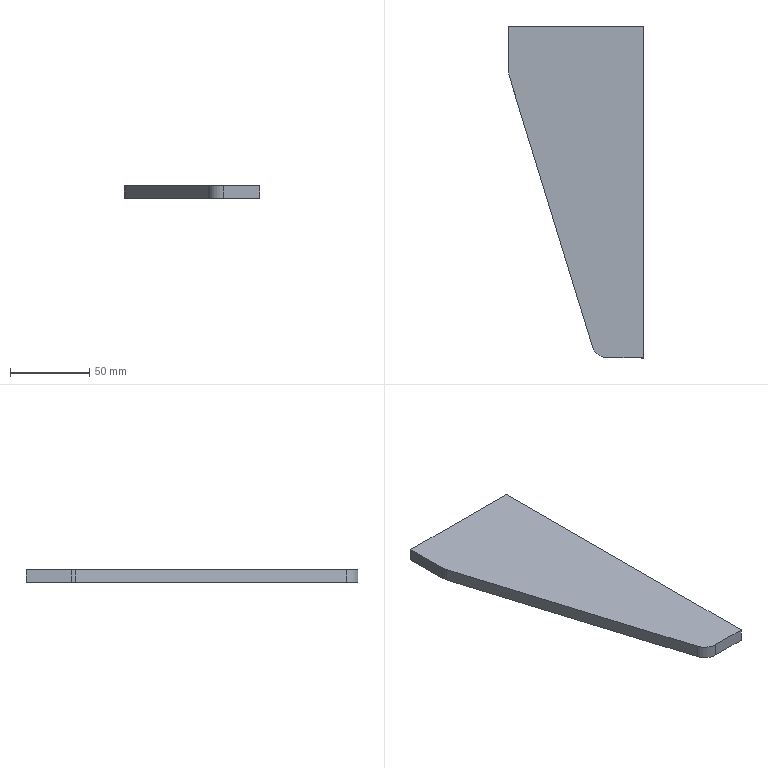Part | SolidWorks | features FlatPattern 1, SMBaseFlange 1, SheetMetal 1 | 1 solid | 9 faces | box 85 x 209 x 8 mm | volume 102657 mm3 | plane 7 | cylinder 2 | commonest cylinder face diameters 20 x2
STEP:
#1=CARTESIAN_POINT('',(-211.101,-990.506,0.));
#2=VERTEX_POINT('',#1);
#3=CARTESIAN_POINT('',(-296.101,-990.506,0.));
#4=VERTEX_POINT('',#3);
#5=CARTESIAN_POINT('',(-296.101,-990.506,0.));
#6=DIRECTION('',(-1.,0.,0.));
#7=VECTOR('',#6,1000.);
#8=LINE('',#5,#7);
#9=EDGE_CURVE('',#2,#4,#8,.T.);
#10=ORIENTED_EDGE('',*,*,#9,.F.);
#11=CARTESIAN_POINT('',(-211.101,-990.506,-8.));
#12=VERTEX_POINT('',#11);
#13=CARTESIAN_POINT('',(-211.101,-990.506,-8.));
#14=DIRECTION('',(0.,0.,1.));
#15=VECTOR('',#14,1000.);
#16=LINE('',#13,#15);
#17=EDGE_CURVE('',#12,#2,#16,.T.);
#18=ORIENTED_EDGE('',*,*,#17,.F.);
#19=CARTESIAN_POINT('',(-296.101,-990.506,-8.));
#20=VERTEX_POINT('',#19);
#21=CARTESIAN_POINT('',(-296.101,-990.506,-8.));
#22=DIRECTION('',(-1.,0.,0.));
#23=VECTOR('',#22,1000.);
#24=LINE('',#21,#23);
#25=EDGE_CURVE('',#12,#20,#24,.T.);
#26=ORIENTED_EDGE('',*,*,#25,.T.);
#27=CARTESIAN_POINT('',(-296.101,-990.506,-8.));
#28=DIRECTION('',(0.,0.,1.));
#29=VECTOR('',#28,1000.);
#30=LINE('',#27,#29);
#31=EDGE_CURVE('',#20,#4,#30,.T.);
#32=ORIENTED_EDGE('',*,*,#31,.T.);
#33=EDGE_LOOP('',(#10,#18,#26,#32));
#34=FACE_OUTER_BOUND('',#33,.T.);
#35=CARTESIAN_POINT('',(-296.101,-990.506,-8.));
#36=DIRECTION('',(0.,1.,0.));
#37=DIRECTION('',(-1.,0.,0.));
#38=AXIS2_PLACEMENT_3D('',#35,#36,#37);
#39=PLANE('',#38);
#40=ADVANCED_FACE('',(#34),#39,.T.);
#41=CARTESIAN_POINT('',(-211.101,-1199.506,0.));
#42=VERTEX_POINT('',#41);
#43=CARTESIAN_POINT('',(-211.101,-990.506,0.));
#44=DIRECTION('',(0.,1.,0.));
#45=VECTOR('',#44,1000.);
#46=LINE('',#43,#45);
#47=EDGE_CURVE('',#42,#2,#46,.T.);
#48=ORIENTED_EDGE('',*,*,#47,.F.);
#49=CARTESIAN_POINT('',(-211.101,-1199.506,-8.));
#50=VERTEX_POINT('',#49);
#51=CARTESIAN_POINT('',(-211.101,-1199.506,-8.));
#52=DIRECTION('',(0.,0.,1.));
#53=VECTOR('',#52,1000.);
#54=LINE('',#51,#53);
#55=EDGE_CURVE('',#50,#42,#54,.T.);
#56=ORIENTED_EDGE('',*,*,#55,.F.);
#57=CARTESIAN_POINT('',(-211.101,-990.506,-8.));
#58=DIRECTION('',(0.,1.,0.));
#59=VECTOR('',#58,1000.);
#60=LINE('',#57,#59);
#61=EDGE_CURVE('',#50,#12,#60,.T.);
#62=ORIENTED_EDGE('',*,*,#61,.T.);
#63=ORIENTED_EDGE('',*,*,#17,.T.);
#64=EDGE_LOOP('',(#48,#56,#62,#63));
#65=FACE_OUTER_BOUND('',#64,.T.);
#66=CARTESIAN_POINT('',(-211.101,-990.506,-8.));
#67=DIRECTION('',(1.,0.,0.));
#68=DIRECTION('',(0.,0.,-1.));
#69=AXIS2_PLACEMENT_3D('',#66,#67,#68);
#70=PLANE('',#69);
#71=ADVANCED_FACE('',(#65),#70,.T.);
#72=CARTESIAN_POINT('',(-233.712,-1199.506,0.));
#73=VERTEX_POINT('',#72);
#74=CARTESIAN_POINT('',(-211.101,-1199.506,0.));
#75=DIRECTION('',(1.,0.,0.));
#76=VECTOR('',#75,1000.);
#77=LINE('',#74,#76);
#78=EDGE_CURVE('',#73,#42,#77,.T.);
#79=ORIENTED_EDGE('',*,*,#78,.F.);
#80=CARTESIAN_POINT('',(-233.712,-1199.506,-8.));
#81=VERTEX_POINT('',#80);
#82=CARTESIAN_POINT('',(-233.712,-1199.506,-8.));
#83=DIRECTION('',(0.,0.,1.));
#84=VECTOR('',#83,1000.);
#85=LINE('',#82,#84);
#86=EDGE_CURVE('',#81,#73,#85,.T.);
#87=ORIENTED_EDGE('',*,*,#86,.F.);
#88=CARTESIAN_POINT('',(-211.101,-1199.506,-8.));
#89=DIRECTION('',(1.,0.,0.));
#90=VECTOR('',#89,1000.);
#91=LINE('',#88,#90);
#92=EDGE_CURVE('',#81,#50,#91,.T.);
#93=ORIENTED_EDGE('',*,*,#92,.T.);
#94=ORIENTED_EDGE('',*,*,#55,.T.);
#95=EDGE_LOOP('',(#79,#87,#93,#94));
#96=FACE_OUTER_BOUND('',#95,.T.);
#97=CARTESIAN_POINT('',(-211.101,-1199.506,-8.));
#98=DIRECTION('',(0.,-1.,0.));
#99=DIRECTION('',(1.,0.,0.));
#100=AXIS2_PLACEMENT_3D('',#97,#98,#99);
#101=PLANE('',#100);
#102=ADVANCED_FACE('',(#96),#101,.T.);
#103=CARTESIAN_POINT('',(-243.271,-1192.443,0.));
#104=VERTEX_POINT('',#103);
#105=CARTESIAN_POINT('',(-233.712,-1189.506,0.));
#106=DIRECTION('',(0.,0.,1.));
#107=DIRECTION('',(-1.,0.,0.));
#108=AXIS2_PLACEMENT_3D('',#105,#106,#107);
#109=CIRCLE('',#108,10.);
#110=EDGE_CURVE('',#104,#73,#109,.T.);
#111=ORIENTED_EDGE('',*,*,#110,.F.);
#112=CARTESIAN_POINT('',(-243.271,-1192.443,-8.));
#113=VERTEX_POINT('',#112);
#114=CARTESIAN_POINT('',(-243.271,-1192.443,-8.));
#115=DIRECTION('',(0.,0.,1.));
#116=VECTOR('',#115,1000.);
#117=LINE('',#114,#116);
#118=EDGE_CURVE('',#113,#104,#117,.T.);
#119=ORIENTED_EDGE('',*,*,#118,.F.);
#120=CARTESIAN_POINT('',(-233.712,-1189.506,-8.));
#121=DIRECTION('',(0.,0.,1.));
#122=DIRECTION('',(-1.,0.,0.));
#123=AXIS2_PLACEMENT_3D('',#120,#121,#122);
#124=CIRCLE('',#123,10.);
#125=EDGE_CURVE('',#113,#81,#124,.T.);
#126=ORIENTED_EDGE('',*,*,#125,.T.);
#127=ORIENTED_EDGE('',*,*,#86,.T.);
#128=EDGE_LOOP('',(#111,#119,#126,#127));
#129=FACE_OUTER_BOUND('',#128,.T.);
#130=CARTESIAN_POINT('',(-233.712,-1189.506,-8.));
#131=DIRECTION('',(0.,0.,1.));
#132=DIRECTION('',(1.,0.,0.));
#133=AXIS2_PLACEMENT_3D('',#130,#131,#132);
#134=CYLINDRICAL_SURFACE('',#133,10.);
#135=ADVANCED_FACE('',(#129),#134,.T.);
#136=CARTESIAN_POINT('',(-295.66,-1021.941,0.));
#137=VERTEX_POINT('',#136);
#138=CARTESIAN_POINT('',(-243.271,-1192.443,0.));
#139=DIRECTION('',(0.2937,-0.9559,0.));
#140=VECTOR('',#139,1000.);
#141=LINE('',#138,#140);
#142=EDGE_CURVE('',#137,#104,#141,.T.);
#143=ORIENTED_EDGE('',*,*,#142,.F.);
#144=CARTESIAN_POINT('',(-295.66,-1021.941,-8.));
#145=VERTEX_POINT('',#144);
#146=CARTESIAN_POINT('',(-295.66,-1021.941,-8.));
#147=DIRECTION('',(0.,0.,1.));
#148=VECTOR('',#147,1000.);
#149=LINE('',#146,#148);
#150=EDGE_CURVE('',#145,#137,#149,.T.);
#151=ORIENTED_EDGE('',*,*,#150,.F.);
#152=CARTESIAN_POINT('',(-243.271,-1192.443,-8.));
#153=DIRECTION('',(0.2937,-0.9559,0.));
#154=VECTOR('',#153,1000.);
#155=LINE('',#152,#154);
#156=EDGE_CURVE('',#145,#113,#155,.T.);
#157=ORIENTED_EDGE('',*,*,#156,.T.);
#158=ORIENTED_EDGE('',*,*,#118,.T.);
#159=EDGE_LOOP('',(#143,#151,#157,#158));
#160=FACE_OUTER_BOUND('',#159,.T.);
#161=CARTESIAN_POINT('',(-243.271,-1192.443,-8.));
#162=DIRECTION('',(-0.9559,-0.2937,0.));
#163=DIRECTION('',(0.2937,-0.9559,0.));
#164=AXIS2_PLACEMENT_3D('',#161,#162,#163);
#165=PLANE('',#164);
#166=ADVANCED_FACE('',(#160),#165,.T.);
#167=CARTESIAN_POINT('',(-296.101,-1019.004,0.));
#168=VERTEX_POINT('',#167);
#169=CARTESIAN_POINT('',(-286.101,-1019.004,0.));
#170=DIRECTION('',(0.,0.,1.));
#171=DIRECTION('',(-1.,0.,0.));
#172=AXIS2_PLACEMENT_3D('',#169,#170,#171);
#173=CIRCLE('',#172,10.);
#174=EDGE_CURVE('',#168,#137,#173,.T.);
#175=ORIENTED_EDGE('',*,*,#174,.F.);
#176=CARTESIAN_POINT('',(-296.101,-1019.004,-8.));
#177=VERTEX_POINT('',#176);
#178=CARTESIAN_POINT('',(-296.101,-1019.004,-8.));
#179=DIRECTION('',(0.,0.,1.));
#180=VECTOR('',#179,1000.);
#181=LINE('',#178,#180);
#182=EDGE_CURVE('',#177,#168,#181,.T.);
#183=ORIENTED_EDGE('',*,*,#182,.F.);
#184=CARTESIAN_POINT('',(-286.101,-1019.004,-8.));
#185=DIRECTION('',(0.,0.,1.));
#186=DIRECTION('',(-1.,0.,0.));
#187=AXIS2_PLACEMENT_3D('',#184,#185,#186);
#188=CIRCLE('',#187,10.);
#189=EDGE_CURVE('',#177,#145,#188,.T.);
#190=ORIENTED_EDGE('',*,*,#189,.T.);
#191=ORIENTED_EDGE('',*,*,#150,.T.);
#192=EDGE_LOOP('',(#175,#183,#190,#191));
#193=FACE_OUTER_BOUND('',#192,.T.);
#194=CARTESIAN_POINT('',(-286.101,-1019.004,-8.));
#195=DIRECTION('',(0.,0.,1.));
#196=DIRECTION('',(1.,0.,0.));
#197=AXIS2_PLACEMENT_3D('',#194,#195,#196);
#198=CYLINDRICAL_SURFACE('',#197,10.);
#199=ADVANCED_FACE('',(#193),#198,.T.);
#200=CARTESIAN_POINT('',(-296.101,-1019.004,0.));
#201=DIRECTION('',(0.,-1.,0.));
#202=VECTOR('',#201,1000.);
#203=LINE('',#200,#202);
#204=EDGE_CURVE('',#4,#168,#203,.T.);
#205=ORIENTED_EDGE('',*,*,#204,.F.);
#206=ORIENTED_EDGE('',*,*,#31,.F.);
#207=CARTESIAN_POINT('',(-296.101,-1019.004,-8.));
#208=DIRECTION('',(0.,-1.,0.));
#209=VECTOR('',#208,1000.);
#210=LINE('',#207,#209);
#211=EDGE_CURVE('',#20,#177,#210,.T.);
#212=ORIENTED_EDGE('',*,*,#211,.T.);
#213=ORIENTED_EDGE('',*,*,#182,.T.);
#214=EDGE_LOOP('',(#205,#206,#212,#213));
#215=FACE_OUTER_BOUND('',#214,.T.);
#216=CARTESIAN_POINT('',(-296.101,-1019.004,-8.));
#217=DIRECTION('',(-1.,0.,0.));
#218=DIRECTION('',(0.,-1.,0.));
#219=AXIS2_PLACEMENT_3D('',#216,#217,#218);
#220=PLANE('',#219);
#221=ADVANCED_FACE('',(#215),#220,.T.);
#222=ORIENTED_EDGE('',*,*,#25,.F.);
#223=ORIENTED_EDGE('',*,*,#61,.F.);
#224=ORIENTED_EDGE('',*,*,#92,.F.);
#225=ORIENTED_EDGE('',*,*,#125,.F.);
#226=ORIENTED_EDGE('',*,*,#156,.F.);
#227=ORIENTED_EDGE('',*,*,#189,.F.);
#228=ORIENTED_EDGE('',*,*,#211,.F.);
#229=EDGE_LOOP('',(#222,#223,#224,#225,#226,#227,#228));
#230=FACE_OUTER_BOUND('',#229,.T.);
#231=CARTESIAN_POINT('',(-233.712,-1189.506,-8.));
#232=DIRECTION('',(0.,0.,-1.));
#233=DIRECTION('',(-1.,0.,0.));
#234=AXIS2_PLACEMENT_3D('',#231,#232,#233);
#235=PLANE('',#234);
#236=ADVANCED_FACE('',(#230),#235,.T.);
#237=ORIENTED_EDGE('',*,*,#9,.T.);
#238=ORIENTED_EDGE('',*,*,#204,.T.);
#239=ORIENTED_EDGE('',*,*,#174,.T.);
#240=ORIENTED_EDGE('',*,*,#142,.T.);
#241=ORIENTED_EDGE('',*,*,#110,.T.);
#242=ORIENTED_EDGE('',*,*,#78,.T.);
#243=ORIENTED_EDGE('',*,*,#47,.T.);
#244=EDGE_LOOP('',(#237,#238,#239,#240,#241,#242,#243));
#245=FACE_OUTER_BOUND('',#244,.T.);
#246=CARTESIAN_POINT('',(-233.712,-1189.506,0.));
#247=DIRECTION('',(0.,0.,-1.));
#248=DIRECTION('',(-1.,0.,0.));
#249=AXIS2_PLACEMENT_3D('',#246,#247,#248);
#250=PLANE('',#249);
#251=ADVANCED_FACE('',(#245),#250,.F.);
#252=CLOSED_SHELL('',(#40,#71,#102,#135,#166,#199,#221,#236,#251));
#253=MANIFOLD_SOLID_BREP('',#252);
#254=CARTESIAN_POINT('',(0.,0.,0.));
#255=DIRECTION('',(0.,0.,1.));
#256=DIRECTION('',(1.,0.,0.));
#257=AXIS2_PLACEMENT_3D('',#254,#255,#256);
#258=(LENGTH_UNIT()NAMED_UNIT(*)SI_UNIT(.MILLI.,.METRE.));
#259=UNCERTAINTY_MEASURE_WITH_UNIT(LENGTH_MEASURE(0.00001),#258,'','');
#260=(NAMED_UNIT(*)PLANE_ANGLE_UNIT()SI_UNIT($,.RADIAN.));
#261=(NAMED_UNIT(*)SI_UNIT($,.STERADIAN.)SOLID_ANGLE_UNIT());
#262=(GEOMETRIC_REPRESENTATION_CONTEXT(3)GLOBAL_UNCERTAINTY_ASSIGNED_CONTEXT((#259))GLOBAL_UNIT_ASSIGNED_CONTEXT((#258,#260,#261))REPRESENTATION_CONTEXT('',''));
#263=ADVANCED_BREP_SHAPE_REPRESENTATION('',(#253,#257),#262);